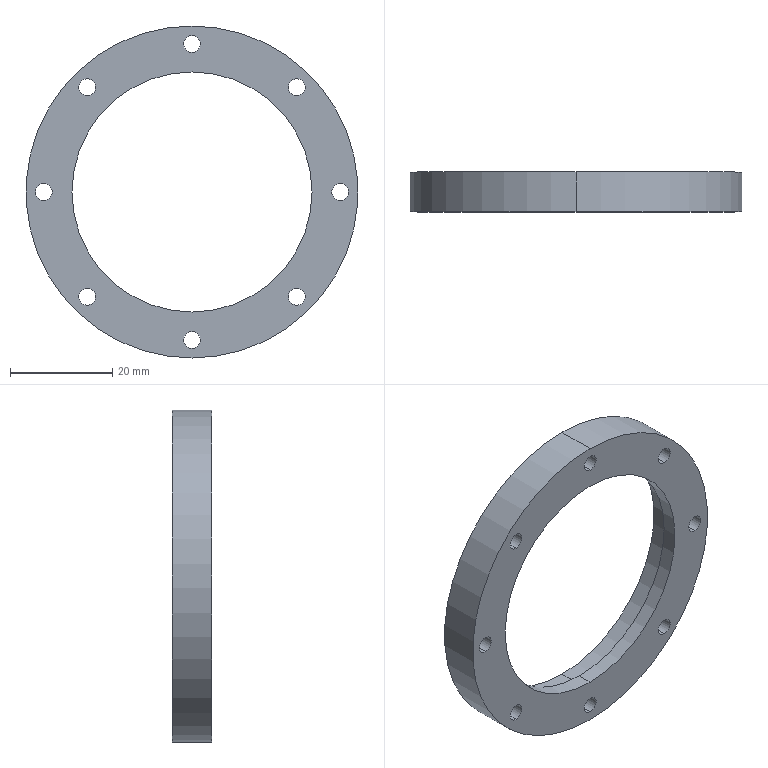Part | SolidWorks | features Extrusion 1, HoleWzd 1, ICE 1 | 1 solid | 25 faces | box 65 x 7.8 x 65 mm | volume 10339 mm3 | cylinder 22 | plane 3 | commonest cylinder face diameters 3.3 x16 47 x2 51 x2 65 x2
STEP:
#1=CARTESIAN_POINT('',(0.,0.,-30.65));
#2=VERTEX_POINT('',#1);
#3=CARTESIAN_POINT('',(0.,0.,-27.35));
#4=VERTEX_POINT('',#3);
#5=CARTESIAN_POINT('',(0.,0.,-29.));
#6=DIRECTION('',(0.,1.,0.));
#7=DIRECTION('',(0.,0.,1.));
#8=AXIS2_PLACEMENT_3D('',#5,#6,#7);
#9=CIRCLE('',#8,1.65);
#10=EDGE_CURVE('',#2,#4,#9,.T.);
#11=ORIENTED_EDGE('',*,*,#10,.F.);
#12=CARTESIAN_POINT('',(0.,7.8,-30.65));
#13=VERTEX_POINT('',#12);
#14=CARTESIAN_POINT('',(0.,7.8,-30.65));
#15=DIRECTION('',(0.,1.,0.));
#16=VECTOR('',#15,1000.);
#17=LINE('',#14,#16);
#18=EDGE_CURVE('',#2,#13,#17,.T.);
#19=ORIENTED_EDGE('',*,*,#18,.T.);
#20=CARTESIAN_POINT('',(0.,7.8,-27.35));
#21=VERTEX_POINT('',#20);
#22=CARTESIAN_POINT('',(0.,7.8,-29.));
#23=DIRECTION('',(0.,1.,0.));
#24=DIRECTION('',(0.,0.,1.));
#25=AXIS2_PLACEMENT_3D('',#22,#23,#24);
#26=CIRCLE('',#25,1.65);
#27=EDGE_CURVE('',#13,#21,#26,.T.);
#28=ORIENTED_EDGE('',*,*,#27,.T.);
#29=CARTESIAN_POINT('',(0.,7.8,-27.35));
#30=DIRECTION('',(0.,1.,0.));
#31=VECTOR('',#30,1000.);
#32=LINE('',#29,#31);
#33=EDGE_CURVE('',#4,#21,#32,.T.);
#34=ORIENTED_EDGE('',*,*,#33,.F.);
#35=EDGE_LOOP('',(#11,#19,#28,#34));
#36=FACE_OUTER_BOUND('',#35,.T.);
#37=CARTESIAN_POINT('',(0.,7.8,-29.));
#38=DIRECTION('',(0.,1.,0.));
#39=DIRECTION('',(0.,0.,1.));
#40=AXIS2_PLACEMENT_3D('',#37,#38,#39);
#41=CYLINDRICAL_SURFACE('',#40,1.65);
#42=ADVANCED_FACE('',(#36),#41,.F.);
#43=CARTESIAN_POINT('',(20.506,0.,-22.156));
#44=VERTEX_POINT('',#43);
#45=CARTESIAN_POINT('',(20.506,0.,-18.856));
#46=VERTEX_POINT('',#45);
#47=CARTESIAN_POINT('',(20.506,0.,-20.506));
#48=DIRECTION('',(0.,1.,0.));
#49=DIRECTION('',(0.,0.,1.));
#50=AXIS2_PLACEMENT_3D('',#47,#48,#49);
#51=CIRCLE('',#50,1.65);
#52=EDGE_CURVE('',#44,#46,#51,.T.);
#53=ORIENTED_EDGE('',*,*,#52,.F.);
#54=CARTESIAN_POINT('',(20.506,7.8,-22.156));
#55=VERTEX_POINT('',#54);
#56=CARTESIAN_POINT('',(20.506,7.8,-22.156));
#57=DIRECTION('',(0.,1.,0.));
#58=VECTOR('',#57,1000.);
#59=LINE('',#56,#58);
#60=EDGE_CURVE('',#44,#55,#59,.T.);
#61=ORIENTED_EDGE('',*,*,#60,.T.);
#62=CARTESIAN_POINT('',(20.506,7.8,-18.856));
#63=VERTEX_POINT('',#62);
#64=CARTESIAN_POINT('',(20.506,7.8,-20.506));
#65=DIRECTION('',(0.,1.,0.));
#66=DIRECTION('',(0.,0.,1.));
#67=AXIS2_PLACEMENT_3D('',#64,#65,#66);
#68=CIRCLE('',#67,1.65);
#69=EDGE_CURVE('',#55,#63,#68,.T.);
#70=ORIENTED_EDGE('',*,*,#69,.T.);
#71=CARTESIAN_POINT('',(20.506,7.8,-18.856));
#72=DIRECTION('',(0.,1.,0.));
#73=VECTOR('',#72,1000.);
#74=LINE('',#71,#73);
#75=EDGE_CURVE('',#46,#63,#74,.T.);
#76=ORIENTED_EDGE('',*,*,#75,.F.);
#77=EDGE_LOOP('',(#53,#61,#70,#76));
#78=FACE_OUTER_BOUND('',#77,.T.);
#79=CARTESIAN_POINT('',(20.506,7.8,-20.506));
#80=DIRECTION('',(0.,1.,0.));
#81=DIRECTION('',(0.,0.,1.));
#82=AXIS2_PLACEMENT_3D('',#79,#80,#81);
#83=CYLINDRICAL_SURFACE('',#82,1.65);
#84=ADVANCED_FACE('',(#78),#83,.F.);
#85=CARTESIAN_POINT('',(29.,0.,-1.65));
#86=VERTEX_POINT('',#85);
#87=CARTESIAN_POINT('',(29.,0.,1.65));
#88=VERTEX_POINT('',#87);
#89=CARTESIAN_POINT('',(29.,0.,0.));
#90=DIRECTION('',(0.,1.,0.));
#91=DIRECTION('',(0.,0.,1.));
#92=AXIS2_PLACEMENT_3D('',#89,#90,#91);
#93=CIRCLE('',#92,1.65);
#94=EDGE_CURVE('',#86,#88,#93,.T.);
#95=ORIENTED_EDGE('',*,*,#94,.F.);
#96=CARTESIAN_POINT('',(29.,7.8,-1.65));
#97=VERTEX_POINT('',#96);
#98=CARTESIAN_POINT('',(29.,7.8,-1.65));
#99=DIRECTION('',(0.,1.,0.));
#100=VECTOR('',#99,1000.);
#101=LINE('',#98,#100);
#102=EDGE_CURVE('',#86,#97,#101,.T.);
#103=ORIENTED_EDGE('',*,*,#102,.T.);
#104=CARTESIAN_POINT('',(29.,7.8,1.65));
#105=VERTEX_POINT('',#104);
#106=CARTESIAN_POINT('',(29.,7.8,0.));
#107=DIRECTION('',(0.,1.,0.));
#108=DIRECTION('',(0.,0.,1.));
#109=AXIS2_PLACEMENT_3D('',#106,#107,#108);
#110=CIRCLE('',#109,1.65);
#111=EDGE_CURVE('',#97,#105,#110,.T.);
#112=ORIENTED_EDGE('',*,*,#111,.T.);
#113=CARTESIAN_POINT('',(29.,7.8,1.65));
#114=DIRECTION('',(0.,1.,0.));
#115=VECTOR('',#114,1000.);
#116=LINE('',#113,#115);
#117=EDGE_CURVE('',#88,#105,#116,.T.);
#118=ORIENTED_EDGE('',*,*,#117,.F.);
#119=EDGE_LOOP('',(#95,#103,#112,#118));
#120=FACE_OUTER_BOUND('',#119,.T.);
#121=CARTESIAN_POINT('',(29.,7.8,0.));
#122=DIRECTION('',(0.,1.,0.));
#123=DIRECTION('',(0.,0.,1.));
#124=AXIS2_PLACEMENT_3D('',#121,#122,#123);
#125=CYLINDRICAL_SURFACE('',#124,1.65);
#126=ADVANCED_FACE('',(#120),#125,.F.);
#127=CARTESIAN_POINT('',(20.506,0.,18.856));
#128=VERTEX_POINT('',#127);
#129=CARTESIAN_POINT('',(20.506,0.,22.156));
#130=VERTEX_POINT('',#129);
#131=CARTESIAN_POINT('',(20.506,0.,20.506));
#132=DIRECTION('',(0.,1.,0.));
#133=DIRECTION('',(0.,0.,1.));
#134=AXIS2_PLACEMENT_3D('',#131,#132,#133);
#135=CIRCLE('',#134,1.65);
#136=EDGE_CURVE('',#128,#130,#135,.T.);
#137=ORIENTED_EDGE('',*,*,#136,.F.);
#138=CARTESIAN_POINT('',(20.506,7.8,18.856));
#139=VERTEX_POINT('',#138);
#140=CARTESIAN_POINT('',(20.506,7.8,18.856));
#141=DIRECTION('',(0.,1.,0.));
#142=VECTOR('',#141,1000.);
#143=LINE('',#140,#142);
#144=EDGE_CURVE('',#128,#139,#143,.T.);
#145=ORIENTED_EDGE('',*,*,#144,.T.);
#146=CARTESIAN_POINT('',(20.506,7.8,22.156));
#147=VERTEX_POINT('',#146);
#148=CARTESIAN_POINT('',(20.506,7.8,20.506));
#149=DIRECTION('',(0.,1.,0.));
#150=DIRECTION('',(0.,0.,1.));
#151=AXIS2_PLACEMENT_3D('',#148,#149,#150);
#152=CIRCLE('',#151,1.65);
#153=EDGE_CURVE('',#139,#147,#152,.T.);
#154=ORIENTED_EDGE('',*,*,#153,.T.);
#155=CARTESIAN_POINT('',(20.506,7.8,22.156));
#156=DIRECTION('',(0.,1.,0.));
#157=VECTOR('',#156,1000.);
#158=LINE('',#155,#157);
#159=EDGE_CURVE('',#130,#147,#158,.T.);
#160=ORIENTED_EDGE('',*,*,#159,.F.);
#161=EDGE_LOOP('',(#137,#145,#154,#160));
#162=FACE_OUTER_BOUND('',#161,.T.);
#163=CARTESIAN_POINT('',(20.506,7.8,20.506));
#164=DIRECTION('',(0.,1.,0.));
#165=DIRECTION('',(0.,0.,1.));
#166=AXIS2_PLACEMENT_3D('',#163,#164,#165);
#167=CYLINDRICAL_SURFACE('',#166,1.65);
#168=ADVANCED_FACE('',(#162),#167,.F.);
#169=CARTESIAN_POINT('',(0.,0.,27.35));
#170=VERTEX_POINT('',#169);
#171=CARTESIAN_POINT('',(0.,0.,30.65));
#172=VERTEX_POINT('',#171);
#173=CARTESIAN_POINT('',(0.,0.,29.));
#174=DIRECTION('',(0.,1.,0.));
#175=DIRECTION('',(0.,0.,1.));
#176=AXIS2_PLACEMENT_3D('',#173,#174,#175);
#177=CIRCLE('',#176,1.65);
#178=EDGE_CURVE('',#170,#172,#177,.T.);
#179=ORIENTED_EDGE('',*,*,#178,.F.);
#180=CARTESIAN_POINT('',(0.,7.8,27.35));
#181=VERTEX_POINT('',#180);
#182=CARTESIAN_POINT('',(0.,7.8,27.35));
#183=DIRECTION('',(0.,1.,0.));
#184=VECTOR('',#183,1000.);
#185=LINE('',#182,#184);
#186=EDGE_CURVE('',#170,#181,#185,.T.);
#187=ORIENTED_EDGE('',*,*,#186,.T.);
#188=CARTESIAN_POINT('',(0.,7.8,30.65));
#189=VERTEX_POINT('',#188);
#190=CARTESIAN_POINT('',(0.,7.8,29.));
#191=DIRECTION('',(0.,1.,0.));
#192=DIRECTION('',(0.,0.,1.));
#193=AXIS2_PLACEMENT_3D('',#190,#191,#192);
#194=CIRCLE('',#193,1.65);
#195=EDGE_CURVE('',#181,#189,#194,.T.);
#196=ORIENTED_EDGE('',*,*,#195,.T.);
#197=CARTESIAN_POINT('',(0.,7.8,30.65));
#198=DIRECTION('',(0.,1.,0.));
#199=VECTOR('',#198,1000.);
#200=LINE('',#197,#199);
#201=EDGE_CURVE('',#172,#189,#200,.T.);
#202=ORIENTED_EDGE('',*,*,#201,.F.);
#203=EDGE_LOOP('',(#179,#187,#196,#202));
#204=FACE_OUTER_BOUND('',#203,.T.);
#205=CARTESIAN_POINT('',(0.,7.8,29.));
#206=DIRECTION('',(0.,1.,0.));
#207=DIRECTION('',(0.,0.,1.));
#208=AXIS2_PLACEMENT_3D('',#205,#206,#207);
#209=CYLINDRICAL_SURFACE('',#208,1.65);
#210=ADVANCED_FACE('',(#204),#209,.F.);
#211=CARTESIAN_POINT('',(-20.506,0.,18.856));
#212=VERTEX_POINT('',#211);
#213=CARTESIAN_POINT('',(-20.506,0.,22.156));
#214=VERTEX_POINT('',#213);
#215=CARTESIAN_POINT('',(-20.506,0.,20.506));
#216=DIRECTION('',(0.,1.,0.));
#217=DIRECTION('',(0.,0.,1.));
#218=AXIS2_PLACEMENT_3D('',#215,#216,#217);
#219=CIRCLE('',#218,1.65);
#220=EDGE_CURVE('',#212,#214,#219,.T.);
#221=ORIENTED_EDGE('',*,*,#220,.F.);
#222=CARTESIAN_POINT('',(-20.506,7.8,18.856));
#223=VERTEX_POINT('',#222);
#224=CARTESIAN_POINT('',(-20.506,7.8,18.856));
#225=DIRECTION('',(0.,1.,0.));
#226=VECTOR('',#225,1000.);
#227=LINE('',#224,#226);
#228=EDGE_CURVE('',#212,#223,#227,.T.);
#229=ORIENTED_EDGE('',*,*,#228,.T.);
#230=CARTESIAN_POINT('',(-20.506,7.8,22.156));
#231=VERTEX_POINT('',#230);
#232=CARTESIAN_POINT('',(-20.506,7.8,20.506));
#233=DIRECTION('',(0.,1.,0.));
#234=DIRECTION('',(0.,0.,1.));
#235=AXIS2_PLACEMENT_3D('',#232,#233,#234);
#236=CIRCLE('',#235,1.65);
#237=EDGE_CURVE('',#223,#231,#236,.T.);
#238=ORIENTED_EDGE('',*,*,#237,.T.);
#239=CARTESIAN_POINT('',(-20.506,7.8,22.156));
#240=DIRECTION('',(0.,1.,0.));
#241=VECTOR('',#240,1000.);
#242=LINE('',#239,#241);
#243=EDGE_CURVE('',#214,#231,#242,.T.);
#244=ORIENTED_EDGE('',*,*,#243,.F.);
#245=EDGE_LOOP('',(#221,#229,#238,#244));
#246=FACE_OUTER_BOUND('',#245,.T.);
#247=CARTESIAN_POINT('',(-20.506,7.8,20.506));
#248=DIRECTION('',(0.,1.,0.));
#249=DIRECTION('',(0.,0.,1.));
#250=AXIS2_PLACEMENT_3D('',#247,#248,#249);
#251=CYLINDRICAL_SURFACE('',#250,1.65);
#252=ADVANCED_FACE('',(#246),#251,.F.);
#253=CARTESIAN_POINT('',(-29.,0.,-1.65));
#254=VERTEX_POINT('',#253);
#255=CARTESIAN_POINT('',(-29.,0.,1.65));
#256=VERTEX_POINT('',#255);
#257=CARTESIAN_POINT('',(-29.,0.,0.));
#258=DIRECTION('',(0.,1.,0.));
#259=DIRECTION('',(0.,0.,1.));
#260=AXIS2_PLACEMENT_3D('',#257,#258,#259);
#261=CIRCLE('',#260,1.65);
#262=EDGE_CURVE('',#254,#256,#261,.T.);
#263=ORIENTED_EDGE('',*,*,#262,.F.);
#264=CARTESIAN_POINT('',(-29.,7.8,-1.65));
#265=VERTEX_POINT('',#264);
#266=CARTESIAN_POINT('',(-29.,7.8,-1.65));
#267=DIRECTION('',(0.,1.,0.));
#268=VECTOR('',#267,1000.);
#269=LINE('',#266,#268);
#270=EDGE_CURVE('',#254,#265,#269,.T.);
#271=ORIENTED_EDGE('',*,*,#270,.T.);
#272=CARTESIAN_POINT('',(-29.,7.8,1.65));
#273=VERTEX_POINT('',#272);
#274=CARTESIAN_POINT('',(-29.,7.8,0.));
#275=DIRECTION('',(0.,1.,0.));
#276=DIRECTION('',(0.,0.,1.));
#277=AXIS2_PLACEMENT_3D('',#274,#275,#276);
#278=CIRCLE('',#277,1.65);
#279=EDGE_CURVE('',#265,#273,#278,.T.);
#280=ORIENTED_EDGE('',*,*,#279,.T.);
#281=CARTESIAN_POINT('',(-29.,7.8,1.65));
#282=DIRECTION('',(0.,1.,0.));
#283=VECTOR('',#282,1000.);
#284=LINE('',#281,#283);
#285=EDGE_CURVE('',#256,#273,#284,.T.);
#286=ORIENTED_EDGE('',*,*,#285,.F.);
#287=EDGE_LOOP('',(#263,#271,#280,#286));
#288=FACE_OUTER_BOUND('',#287,.T.);
#289=CARTESIAN_POINT('',(-29.,7.8,0.));
#290=DIRECTION('',(0.,1.,0.));
#291=DIRECTION('',(0.,0.,1.));
#292=AXIS2_PLACEMENT_3D('',#289,#290,#291);
#293=CYLINDRICAL_SURFACE('',#292,1.65);
#294=ADVANCED_FACE('',(#288),#293,.F.);
#295=CARTESIAN_POINT('',(-20.506,0.,-22.156));
#296=VERTEX_POINT('',#295);
#297=CARTESIAN_POINT('',(-20.506,0.,-18.856));
#298=VERTEX_POINT('',#297);
#299=CARTESIAN_POINT('',(-20.506,0.,-20.506));
#300=DIRECTION('',(0.,1.,0.));
#301=DIRECTION('',(0.,0.,1.));
#302=AXIS2_PLACEMENT_3D('',#299,#300,#301);
#303=CIRCLE('',#302,1.65);
#304=EDGE_CURVE('',#296,#298,#303,.T.);
#305=ORIENTED_EDGE('',*,*,#304,.F.);
#306=CARTESIAN_POINT('',(-20.506,7.8,-22.156));
#307=VERTEX_POINT('',#306);
#308=CARTESIAN_POINT('',(-20.506,7.8,-22.156));
#309=DIRECTION('',(0.,1.,0.));
#310=VECTOR('',#309,1000.);
#311=LINE('',#308,#310);
#312=EDGE_CURVE('',#296,#307,#311,.T.);
#313=ORIENTED_EDGE('',*,*,#312,.T.);
#314=CARTESIAN_POINT('',(-20.506,7.8,-18.856));
#315=VERTEX_POINT('',#314);
#316=CARTESIAN_POINT('',(-20.506,7.8,-20.506));
#317=DIRECTION('',(0.,1.,0.));
#318=DIRECTION('',(0.,0.,1.));
#319=AXIS2_PLACEMENT_3D('',#316,#317,#318);
#320=CIRCLE('',#319,1.65);
#321=EDGE_CURVE('',#307,#315,#320,.T.);
#322=ORIENTED_EDGE('',*,*,#321,.T.);
#323=CARTESIAN_POINT('',(-20.506,7.8,-18.856));
#324=DIRECTION('',(0.,1.,0.));
#325=VECTOR('',#324,1000.);
#326=LINE('',#323,#325);
#327=EDGE_CURVE('',#298,#315,#326,.T.);
#328=ORIENTED_EDGE('',*,*,#327,.F.);
#329=EDGE_LOOP('',(#305,#313,#322,#328));
#330=FACE_OUTER_BOUND('',#329,.T.);
#331=CARTESIAN_POINT('',(-20.506,7.8,-20.506));
#332=DIRECTION('',(0.,1.,0.));
#333=DIRECTION('',(0.,0.,1.));
#334=AXIS2_PLACEMENT_3D('',#331,#332,#333);
#335=CYLINDRICAL_SURFACE('',#334,1.65);
#336=ADVANCED_FACE('',(#330),#335,.F.);
#337=CARTESIAN_POINT('',(0.,7.8,-25.5));
#338=VERTEX_POINT('',#337);
#339=CARTESIAN_POINT('',(0.,7.8,25.5));
#340=VERTEX_POINT('',#339);
#341=CARTESIAN_POINT('',(0.,7.8,0.));
#342=DIRECTION('',(0.,1.,0.));
#343=DIRECTION('',(0.,0.,1.));
#344=AXIS2_PLACEMENT_3D('',#341,#342,#343);
#345=CIRCLE('',#344,25.5);
#346=EDGE_CURVE('',#338,#340,#345,.T.);
#347=ORIENTED_EDGE('',*,*,#346,.T.);
#348=CARTESIAN_POINT('',(0.,3.,25.5));
#349=VERTEX_POINT('',#348);
#350=CARTESIAN_POINT('',(0.,7.8,25.5));
#351=DIRECTION('',(0.,-1.,0.));
#352=VECTOR('',#351,1000.);
#353=LINE('',#350,#352);
#354=EDGE_CURVE('',#340,#349,#353,.T.);
#355=ORIENTED_EDGE('',*,*,#354,.T.);
#356=CARTESIAN_POINT('',(0.,3.,-25.5));
#357=VERTEX_POINT('',#356);
#358=CARTESIAN_POINT('',(0.,3.,0.));
#359=DIRECTION('',(0.,1.,0.));
#360=DIRECTION('',(0.,0.,1.));
#361=AXIS2_PLACEMENT_3D('',#358,#359,#360);
#362=CIRCLE('',#361,25.5);
#363=EDGE_CURVE('',#357,#349,#362,.T.);
#364=ORIENTED_EDGE('',*,*,#363,.F.);
#365=CARTESIAN_POINT('',(0.,7.8,-25.5));
#366=DIRECTION('',(0.,-1.,0.));
#367=VECTOR('',#366,1000.);
#368=LINE('',#365,#367);
#369=EDGE_CURVE('',#338,#357,#368,.T.);
#370=ORIENTED_EDGE('',*,*,#369,.F.);
#371=EDGE_LOOP('',(#347,#355,#364,#370));
#372=FACE_OUTER_BOUND('',#371,.T.);
#373=CARTESIAN_POINT('',(0.,7.8,0.));
#374=DIRECTION('',(0.,-1.,0.));
#375=DIRECTION('',(0.,0.,-1.));
#376=AXIS2_PLACEMENT_3D('',#373,#374,#375);
#377=CYLINDRICAL_SURFACE('',#376,25.5);
#378=ADVANCED_FACE('',(#372),#377,.F.);
#379=CARTESIAN_POINT('',(0.,3.,-23.5));
#380=VERTEX_POINT('',#379);
#381=CARTESIAN_POINT('',(0.,3.,23.5));
#382=VERTEX_POINT('',#381);
#383=CARTESIAN_POINT('',(0.,3.,0.));
#384=DIRECTION('',(0.,1.,0.));
#385=DIRECTION('',(0.,0.,1.));
#386=AXIS2_PLACEMENT_3D('',#383,#384,#385);
#387=CIRCLE('',#386,23.5);
#388=EDGE_CURVE('',#380,#382,#387,.T.);
#389=ORIENTED_EDGE('',*,*,#388,.T.);
#390=CARTESIAN_POINT('',(0.,0.,23.5));
#391=VERTEX_POINT('',#390);
#392=CARTESIAN_POINT('',(0.,3.,23.5));
#393=DIRECTION('',(0.,-1.,0.));
#394=VECTOR('',#393,1000.);
#395=LINE('',#392,#394);
#396=EDGE_CURVE('',#382,#391,#395,.T.);
#397=ORIENTED_EDGE('',*,*,#396,.T.);
#398=CARTESIAN_POINT('',(0.,0.,-23.5));
#399=VERTEX_POINT('',#398);
#400=CARTESIAN_POINT('',(0.,0.,0.));
#401=DIRECTION('',(0.,1.,0.));
#402=DIRECTION('',(0.,0.,1.));
#403=AXIS2_PLACEMENT_3D('',#400,#401,#402);
#404=CIRCLE('',#403,23.5);
#405=EDGE_CURVE('',#399,#391,#404,.T.);
#406=ORIENTED_EDGE('',*,*,#405,.F.);
#407=CARTESIAN_POINT('',(0.,3.,-23.5));
#408=DIRECTION('',(0.,-1.,0.));
#409=VECTOR('',#408,1000.);
#410=LINE('',#407,#409);
#411=EDGE_CURVE('',#380,#399,#410,.T.);
#412=ORIENTED_EDGE('',*,*,#411,.F.);
#413=EDGE_LOOP('',(#389,#397,#406,#412));
#414=FACE_OUTER_BOUND('',#413,.T.);
#415=CARTESIAN_POINT('',(0.,3.,0.));
#416=DIRECTION('',(0.,-1.,0.));
#417=DIRECTION('',(0.,0.,-1.));
#418=AXIS2_PLACEMENT_3D('',#415,#416,#417);
#419=CYLINDRICAL_SURFACE('',#418,23.5);
#420=ADVANCED_FACE('',(#414),#419,.F.);
#421=CARTESIAN_POINT('',(0.,7.8,32.5));
#422=VERTEX_POINT('',#421);
#423=CARTESIAN_POINT('',(0.,7.8,-32.5));
#424=VERTEX_POINT('',#423);
#425=CARTESIAN_POINT('',(0.,7.8,0.));
#426=DIRECTION('',(0.,1.,0.));
#427=DIRECTION('',(0.,0.,1.));
#428=AXIS2_PLACEMENT_3D('',#425,#426,#427);
#429=CIRCLE('',#428,32.5);
#430=EDGE_CURVE('',#422,#424,#429,.T.);
#431=ORIENTED_EDGE('',*,*,#430,.F.);
#432=CARTESIAN_POINT('',(0.,0.,32.5));
#433=VERTEX_POINT('',#432);
#434=CARTESIAN_POINT('',(0.,3.,32.5));
#435=DIRECTION('',(0.,-1.,0.));
#436=VECTOR('',#435,1000.);
#437=LINE('',#434,#436);
#438=EDGE_CURVE('',#422,#433,#437,.T.);
#439=ORIENTED_EDGE('',*,*,#438,.T.);
#440=CARTESIAN_POINT('',(0.,0.,-32.5));
#441=VERTEX_POINT('',#440);
#442=CARTESIAN_POINT('',(0.,0.,0.));
#443=DIRECTION('',(0.,1.,0.));
#444=DIRECTION('',(0.,0.,1.));
#445=AXIS2_PLACEMENT_3D('',#442,#443,#444);
#446=CIRCLE('',#445,32.5);
#447=EDGE_CURVE('',#433,#441,#446,.T.);
#448=ORIENTED_EDGE('',*,*,#447,.T.);
#449=CARTESIAN_POINT('',(0.,3.,-32.5));
#450=DIRECTION('',(0.,-1.,0.));
#451=VECTOR('',#450,1000.);
#452=LINE('',#449,#451);
#453=EDGE_CURVE('',#424,#441,#452,.T.);
#454=ORIENTED_EDGE('',*,*,#453,.F.);
#455=EDGE_LOOP('',(#431,#439,#448,#454));
#456=FACE_OUTER_BOUND('',#455,.T.);
#457=CARTESIAN_POINT('',(0.,3.,0.));
#458=DIRECTION('',(0.,-1.,0.));
#459=DIRECTION('',(0.,0.,-1.));
#460=AXIS2_PLACEMENT_3D('',#457,#458,#459);
#461=CYLINDRICAL_SURFACE('',#460,32.5);
#462=ADVANCED_FACE('',(#456),#461,.T.);
#463=ORIENTED_EDGE('',*,*,#388,.F.);
#464=CARTESIAN_POINT('',(0.,3.,0.));
#465=DIRECTION('',(0.,1.,0.));
#466=DIRECTION('',(0.,0.,1.));
#467=AXIS2_PLACEMENT_3D('',#464,#465,#466);
#468=CIRCLE('',#467,23.5);
#469=EDGE_CURVE('',#382,#380,#468,.T.);
#470=ORIENTED_EDGE('',*,*,#469,.F.);
#471=EDGE_LOOP('',(#463,#470));
#472=FACE_BOUND('',#471,.T.);
#473=ORIENTED_EDGE('',*,*,#363,.T.);
#474=CARTESIAN_POINT('',(0.,3.,0.));
#475=DIRECTION('',(0.,1.,0.));
#476=DIRECTION('',(0.,0.,1.));
#477=AXIS2_PLACEMENT_3D('',#474,#475,#476);
#478=CIRCLE('',#477,25.5);
#479=EDGE_CURVE('',#349,#357,#478,.T.);
#480=ORIENTED_EDGE('',*,*,#479,.T.);
#481=EDGE_LOOP('',(#473,#480));
#482=FACE_OUTER_BOUND('',#481,.T.);
#483=CARTESIAN_POINT('',(0.,3.,0.));
#484=DIRECTION('',(0.,1.,0.));
#485=DIRECTION('',(0.,0.,1.));
#486=AXIS2_PLACEMENT_3D('',#483,#484,#485);
#487=PLANE('',#486);
#488=ADVANCED_FACE('',(#472,#482),#487,.T.);
#489=CARTESIAN_POINT('',(0.,0.,-29.));
#490=DIRECTION('',(0.,1.,0.));
#491=DIRECTION('',(0.,0.,1.));
#492=AXIS2_PLACEMENT_3D('',#489,#490,#491);
#493=CIRCLE('',#492,1.65);
#494=EDGE_CURVE('',#4,#2,#493,.T.);
#495=ORIENTED_EDGE('',*,*,#494,.T.);
#496=ORIENTED_EDGE('',*,*,#10,.T.);
#497=EDGE_LOOP('',(#495,#496));
#498=FACE_BOUND('',#497,.T.);
#499=CARTESIAN_POINT('',(20.506,0.,-20.506));
#500=DIRECTION('',(0.,1.,0.));
#501=DIRECTION('',(0.,0.,1.));
#502=AXIS2_PLACEMENT_3D('',#499,#500,#501);
#503=CIRCLE('',#502,1.65);
#504=EDGE_CURVE('',#46,#44,#503,.T.);
#505=ORIENTED_EDGE('',*,*,#504,.T.);
#506=ORIENTED_EDGE('',*,*,#52,.T.);
#507=EDGE_LOOP('',(#505,#506));
#508=FACE_BOUND('',#507,.T.);
#509=CARTESIAN_POINT('',(29.,0.,0.));
#510=DIRECTION('',(0.,1.,0.));
#511=DIRECTION('',(0.,0.,1.));
#512=AXIS2_PLACEMENT_3D('',#509,#510,#511);
#513=CIRCLE('',#512,1.65);
#514=EDGE_CURVE('',#88,#86,#513,.T.);
#515=ORIENTED_EDGE('',*,*,#514,.T.);
#516=ORIENTED_EDGE('',*,*,#94,.T.);
#517=EDGE_LOOP('',(#515,#516));
#518=FACE_BOUND('',#517,.T.);
#519=CARTESIAN_POINT('',(20.506,0.,20.506));
#520=DIRECTION('',(0.,1.,0.));
#521=DIRECTION('',(0.,0.,1.));
#522=AXIS2_PLACEMENT_3D('',#519,#520,#521);
#523=CIRCLE('',#522,1.65);
#524=EDGE_CURVE('',#130,#128,#523,.T.);
#525=ORIENTED_EDGE('',*,*,#524,.T.);
#526=ORIENTED_EDGE('',*,*,#136,.T.);
#527=EDGE_LOOP('',(#525,#526));
#528=FACE_BOUND('',#527,.T.);
#529=CARTESIAN_POINT('',(0.,0.,29.));
#530=DIRECTION('',(0.,1.,0.));
#531=DIRECTION('',(0.,0.,1.));
#532=AXIS2_PLACEMENT_3D('',#529,#530,#531);
#533=CIRCLE('',#532,1.65);
#534=EDGE_CURVE('',#172,#170,#533,.T.);
#535=ORIENTED_EDGE('',*,*,#534,.T.);
#536=ORIENTED_EDGE('',*,*,#178,.T.);
#537=EDGE_LOOP('',(#535,#536));
#538=FACE_BOUND('',#537,.T.);
#539=CARTESIAN_POINT('',(-20.506,0.,20.506));
#540=DIRECTION('',(0.,1.,0.));
#541=DIRECTION('',(0.,0.,1.));
#542=AXIS2_PLACEMENT_3D('',#539,#540,#541);
#543=CIRCLE('',#542,1.65);
#544=EDGE_CURVE('',#214,#212,#543,.T.);
#545=ORIENTED_EDGE('',*,*,#544,.T.);
#546=ORIENTED_EDGE('',*,*,#220,.T.);
#547=EDGE_LOOP('',(#545,#546));
#548=FACE_BOUND('',#547,.T.);
#549=CARTESIAN_POINT('',(-29.,0.,0.));
#550=DIRECTION('',(0.,1.,0.));
#551=DIRECTION('',(0.,0.,1.));
#552=AXIS2_PLACEMENT_3D('',#549,#550,#551);
#553=CIRCLE('',#552,1.65);
#554=EDGE_CURVE('',#256,#254,#553,.T.);
#555=ORIENTED_EDGE('',*,*,#554,.T.);
#556=ORIENTED_EDGE('',*,*,#262,.T.);
#557=EDGE_LOOP('',(#555,#556));
#558=FACE_BOUND('',#557,.T.);
#559=CARTESIAN_POINT('',(-20.506,0.,-20.506));
#560=DIRECTION('',(0.,1.,0.));
#561=DIRECTION('',(0.,0.,1.));
#562=AXIS2_PLACEMENT_3D('',#559,#560,#561);
#563=CIRCLE('',#562,1.65);
#564=EDGE_CURVE('',#298,#296,#563,.T.);
#565=ORIENTED_EDGE('',*,*,#564,.T.);
#566=ORIENTED_EDGE('',*,*,#304,.T.);
#567=EDGE_LOOP('',(#565,#566));
#568=FACE_BOUND('',#567,.T.);
#569=CARTESIAN_POINT('',(0.,0.,0.));
#570=DIRECTION('',(0.,1.,0.));
#571=DIRECTION('',(0.,0.,1.));
#572=AXIS2_PLACEMENT_3D('',#569,#570,#571);
#573=CIRCLE('',#572,32.5);
#574=EDGE_CURVE('',#441,#433,#573,.T.);
#575=ORIENTED_EDGE('',*,*,#574,.F.);
#576=ORIENTED_EDGE('',*,*,#447,.F.);
#577=EDGE_LOOP('',(#575,#576));
#578=FACE_OUTER_BOUND('',#577,.T.);
#579=ORIENTED_EDGE('',*,*,#405,.T.);
#580=CARTESIAN_POINT('',(0.,0.,0.));
#581=DIRECTION('',(0.,1.,0.));
#582=DIRECTION('',(0.,0.,1.));
#583=AXIS2_PLACEMENT_3D('',#580,#581,#582);
#584=CIRCLE('',#583,23.5);
#585=EDGE_CURVE('',#391,#399,#584,.T.);
#586=ORIENTED_EDGE('',*,*,#585,.T.);
#587=EDGE_LOOP('',(#579,#586));
#588=FACE_BOUND('',#587,.T.);
#589=CARTESIAN_POINT('',(0.,0.,0.));
#590=DIRECTION('',(0.,1.,0.));
#591=DIRECTION('',(0.,0.,1.));
#592=AXIS2_PLACEMENT_3D('',#589,#590,#591);
#593=PLANE('',#592);
#594=ADVANCED_FACE('',(#498,#508,#518,#528,#538,#548,#558,#568,#578,#588),#593,.F.);
#595=ORIENTED_EDGE('',*,*,#438,.F.);
#596=CARTESIAN_POINT('',(0.,7.8,0.));
#597=DIRECTION('',(0.,1.,0.));
#598=DIRECTION('',(0.,0.,1.));
#599=AXIS2_PLACEMENT_3D('',#596,#597,#598);
#600=CIRCLE('',#599,32.5);
#601=EDGE_CURVE('',#424,#422,#600,.T.);
#602=ORIENTED_EDGE('',*,*,#601,.F.);
#603=ORIENTED_EDGE('',*,*,#453,.T.);
#604=ORIENTED_EDGE('',*,*,#574,.T.);
#605=EDGE_LOOP('',(#595,#602,#603,#604));
#606=FACE_OUTER_BOUND('',#605,.T.);
#607=CARTESIAN_POINT('',(0.,3.,0.));
#608=DIRECTION('',(0.,-1.,0.));
#609=DIRECTION('',(0.,0.,-1.));
#610=AXIS2_PLACEMENT_3D('',#607,#608,#609);
#611=CYLINDRICAL_SURFACE('',#610,32.5);
#612=ADVANCED_FACE('',(#606),#611,.T.);
#613=ORIENTED_EDGE('',*,*,#396,.F.);
#614=ORIENTED_EDGE('',*,*,#469,.T.);
#615=ORIENTED_EDGE('',*,*,#411,.T.);
#616=ORIENTED_EDGE('',*,*,#585,.F.);
#617=EDGE_LOOP('',(#613,#614,#615,#616));
#618=FACE_OUTER_BOUND('',#617,.T.);
#619=CARTESIAN_POINT('',(0.,3.,0.));
#620=DIRECTION('',(0.,-1.,0.));
#621=DIRECTION('',(0.,0.,-1.));
#622=AXIS2_PLACEMENT_3D('',#619,#620,#621);
#623=CYLINDRICAL_SURFACE('',#622,23.5);
#624=ADVANCED_FACE('',(#618),#623,.F.);
#625=CARTESIAN_POINT('',(0.,7.8,-29.));
#626=DIRECTION('',(0.,1.,0.));
#627=DIRECTION('',(0.,0.,1.));
#628=AXIS2_PLACEMENT_3D('',#625,#626,#627);
#629=CIRCLE('',#628,1.65);
#630=EDGE_CURVE('',#21,#13,#629,.T.);
#631=ORIENTED_EDGE('',*,*,#630,.F.);
#632=ORIENTED_EDGE('',*,*,#27,.F.);
#633=EDGE_LOOP('',(#631,#632));
#634=FACE_BOUND('',#633,.T.);
#635=CARTESIAN_POINT('',(20.506,7.8,-20.506));
#636=DIRECTION('',(0.,1.,0.));
#637=DIRECTION('',(0.,0.,1.));
#638=AXIS2_PLACEMENT_3D('',#635,#636,#637);
#639=CIRCLE('',#638,1.65);
#640=EDGE_CURVE('',#63,#55,#639,.T.);
#641=ORIENTED_EDGE('',*,*,#640,.F.);
#642=ORIENTED_EDGE('',*,*,#69,.F.);
#643=EDGE_LOOP('',(#641,#642));
#644=FACE_BOUND('',#643,.T.);
#645=CARTESIAN_POINT('',(29.,7.8,0.));
#646=DIRECTION('',(0.,1.,0.));
#647=DIRECTION('',(0.,0.,1.));
#648=AXIS2_PLACEMENT_3D('',#645,#646,#647);
#649=CIRCLE('',#648,1.65);
#650=EDGE_CURVE('',#105,#97,#649,.T.);
#651=ORIENTED_EDGE('',*,*,#650,.F.);
#652=ORIENTED_EDGE('',*,*,#111,.F.);
#653=EDGE_LOOP('',(#651,#652));
#654=FACE_BOUND('',#653,.T.);
#655=CARTESIAN_POINT('',(20.506,7.8,20.506));
#656=DIRECTION('',(0.,1.,0.));
#657=DIRECTION('',(0.,0.,1.));
#658=AXIS2_PLACEMENT_3D('',#655,#656,#657);
#659=CIRCLE('',#658,1.65);
#660=EDGE_CURVE('',#147,#139,#659,.T.);
#661=ORIENTED_EDGE('',*,*,#660,.F.);
#662=ORIENTED_EDGE('',*,*,#153,.F.);
#663=EDGE_LOOP('',(#661,#662));
#664=FACE_BOUND('',#663,.T.);
#665=CARTESIAN_POINT('',(0.,7.8,29.));
#666=DIRECTION('',(0.,1.,0.));
#667=DIRECTION('',(0.,0.,1.));
#668=AXIS2_PLACEMENT_3D('',#665,#666,#667);
#669=CIRCLE('',#668,1.65);
#670=EDGE_CURVE('',#189,#181,#669,.T.);
#671=ORIENTED_EDGE('',*,*,#670,.F.);
#672=ORIENTED_EDGE('',*,*,#195,.F.);
#673=EDGE_LOOP('',(#671,#672));
#674=FACE_BOUND('',#673,.T.);
#675=CARTESIAN_POINT('',(-20.506,7.8,20.506));
#676=DIRECTION('',(0.,1.,0.));
#677=DIRECTION('',(0.,0.,1.));
#678=AXIS2_PLACEMENT_3D('',#675,#676,#677);
#679=CIRCLE('',#678,1.65);
#680=EDGE_CURVE('',#231,#223,#679,.T.);
#681=ORIENTED_EDGE('',*,*,#680,.F.);
#682=ORIENTED_EDGE('',*,*,#237,.F.);
#683=EDGE_LOOP('',(#681,#682));
#684=FACE_BOUND('',#683,.T.);
#685=CARTESIAN_POINT('',(-29.,7.8,0.));
#686=DIRECTION('',(0.,1.,0.));
#687=DIRECTION('',(0.,0.,1.));
#688=AXIS2_PLACEMENT_3D('',#685,#686,#687);
#689=CIRCLE('',#688,1.65);
#690=EDGE_CURVE('',#273,#265,#689,.T.);
#691=ORIENTED_EDGE('',*,*,#690,.F.);
#692=ORIENTED_EDGE('',*,*,#279,.F.);
#693=EDGE_LOOP('',(#691,#692));
#694=FACE_BOUND('',#693,.T.);
#695=CARTESIAN_POINT('',(-20.506,7.8,-20.506));
#696=DIRECTION('',(0.,1.,0.));
#697=DIRECTION('',(0.,0.,1.));
#698=AXIS2_PLACEMENT_3D('',#695,#696,#697);
#699=CIRCLE('',#698,1.65);
#700=EDGE_CURVE('',#315,#307,#699,.T.);
#701=ORIENTED_EDGE('',*,*,#700,.F.);
#702=ORIENTED_EDGE('',*,*,#321,.F.);
#703=EDGE_LOOP('',(#701,#702));
#704=FACE_BOUND('',#703,.T.);
#705=ORIENTED_EDGE('',*,*,#601,.T.);
#706=ORIENTED_EDGE('',*,*,#430,.T.);
#707=EDGE_LOOP('',(#705,#706));
#708=FACE_OUTER_BOUND('',#707,.T.);
#709=ORIENTED_EDGE('',*,*,#346,.F.);
#710=CARTESIAN_POINT('',(0.,7.8,0.));
#711=DIRECTION('',(0.,1.,0.));
#712=DIRECTION('',(0.,0.,1.));
#713=AXIS2_PLACEMENT_3D('',#710,#711,#712);
#714=CIRCLE('',#713,25.5);
#715=EDGE_CURVE('',#340,#338,#714,.T.);
#716=ORIENTED_EDGE('',*,*,#715,.F.);
#717=EDGE_LOOP('',(#709,#716));
#718=FACE_BOUND('',#717,.T.);
#719=CARTESIAN_POINT('',(0.,7.8,0.));
#720=DIRECTION('',(0.,1.,0.));
#721=DIRECTION('',(0.,0.,1.));
#722=AXIS2_PLACEMENT_3D('',#719,#720,#721);
#723=PLANE('',#722);
#724=ADVANCED_FACE('',(#634,#644,#654,#664,#674,#684,#694,#704,#708,#718),#723,.T.);
#725=ORIENTED_EDGE('',*,*,#354,.F.);
#726=ORIENTED_EDGE('',*,*,#715,.T.);
#727=ORIENTED_EDGE('',*,*,#369,.T.);
#728=ORIENTED_EDGE('',*,*,#479,.F.);
#729=EDGE_LOOP('',(#725,#726,#727,#728));
#730=FACE_OUTER_BOUND('',#729,.T.);
#731=CARTESIAN_POINT('',(0.,7.8,0.));
#732=DIRECTION('',(0.,-1.,0.));
#733=DIRECTION('',(0.,0.,-1.));
#734=AXIS2_PLACEMENT_3D('',#731,#732,#733);
#735=CYLINDRICAL_SURFACE('',#734,25.5);
#736=ADVANCED_FACE('',(#730),#735,.F.);
#737=ORIENTED_EDGE('',*,*,#312,.F.);
#738=ORIENTED_EDGE('',*,*,#564,.F.);
#739=ORIENTED_EDGE('',*,*,#327,.T.);
#740=ORIENTED_EDGE('',*,*,#700,.T.);
#741=EDGE_LOOP('',(#737,#738,#739,#740));
#742=FACE_OUTER_BOUND('',#741,.T.);
#743=CARTESIAN_POINT('',(-20.506,7.8,-20.506));
#744=DIRECTION('',(0.,1.,0.));
#745=DIRECTION('',(0.,0.,1.));
#746=AXIS2_PLACEMENT_3D('',#743,#744,#745);
#747=CYLINDRICAL_SURFACE('',#746,1.65);
#748=ADVANCED_FACE('',(#742),#747,.F.);
#749=ORIENTED_EDGE('',*,*,#270,.F.);
#750=ORIENTED_EDGE('',*,*,#554,.F.);
#751=ORIENTED_EDGE('',*,*,#285,.T.);
#752=ORIENTED_EDGE('',*,*,#690,.T.);
#753=EDGE_LOOP('',(#749,#750,#751,#752));
#754=FACE_OUTER_BOUND('',#753,.T.);
#755=CARTESIAN_POINT('',(-29.,7.8,0.));
#756=DIRECTION('',(0.,1.,0.));
#757=DIRECTION('',(0.,0.,1.));
#758=AXIS2_PLACEMENT_3D('',#755,#756,#757);
#759=CYLINDRICAL_SURFACE('',#758,1.65);
#760=ADVANCED_FACE('',(#754),#759,.F.);
#761=ORIENTED_EDGE('',*,*,#228,.F.);
#762=ORIENTED_EDGE('',*,*,#544,.F.);
#763=ORIENTED_EDGE('',*,*,#243,.T.);
#764=ORIENTED_EDGE('',*,*,#680,.T.);
#765=EDGE_LOOP('',(#761,#762,#763,#764));
#766=FACE_OUTER_BOUND('',#765,.T.);
#767=CARTESIAN_POINT('',(-20.506,7.8,20.506));
#768=DIRECTION('',(0.,1.,0.));
#769=DIRECTION('',(0.,0.,1.));
#770=AXIS2_PLACEMENT_3D('',#767,#768,#769);
#771=CYLINDRICAL_SURFACE('',#770,1.65);
#772=ADVANCED_FACE('',(#766),#771,.F.);
#773=ORIENTED_EDGE('',*,*,#186,.F.);
#774=ORIENTED_EDGE('',*,*,#534,.F.);
#775=ORIENTED_EDGE('',*,*,#201,.T.);
#776=ORIENTED_EDGE('',*,*,#670,.T.);
#777=EDGE_LOOP('',(#773,#774,#775,#776));
#778=FACE_OUTER_BOUND('',#777,.T.);
#779=CARTESIAN_POINT('',(0.,7.8,29.));
#780=DIRECTION('',(0.,1.,0.));
#781=DIRECTION('',(0.,0.,1.));
#782=AXIS2_PLACEMENT_3D('',#779,#780,#781);
#783=CYLINDRICAL_SURFACE('',#782,1.65);
#784=ADVANCED_FACE('',(#778),#783,.F.);
#785=ORIENTED_EDGE('',*,*,#144,.F.);
#786=ORIENTED_EDGE('',*,*,#524,.F.);
#787=ORIENTED_EDGE('',*,*,#159,.T.);
#788=ORIENTED_EDGE('',*,*,#660,.T.);
#789=EDGE_LOOP('',(#785,#786,#787,#788));
#790=FACE_OUTER_BOUND('',#789,.T.);
#791=CARTESIAN_POINT('',(20.506,7.8,20.506));
#792=DIRECTION('',(0.,1.,0.));
#793=DIRECTION('',(0.,0.,1.));
#794=AXIS2_PLACEMENT_3D('',#791,#792,#793);
#795=CYLINDRICAL_SURFACE('',#794,1.65);
#796=ADVANCED_FACE('',(#790),#795,.F.);
#797=ORIENTED_EDGE('',*,*,#102,.F.);
#798=ORIENTED_EDGE('',*,*,#514,.F.);
#799=ORIENTED_EDGE('',*,*,#117,.T.);
#800=ORIENTED_EDGE('',*,*,#650,.T.);
#801=EDGE_LOOP('',(#797,#798,#799,#800));
#802=FACE_OUTER_BOUND('',#801,.T.);
#803=CARTESIAN_POINT('',(29.,7.8,0.));
#804=DIRECTION('',(0.,1.,0.));
#805=DIRECTION('',(0.,0.,1.));
#806=AXIS2_PLACEMENT_3D('',#803,#804,#805);
#807=CYLINDRICAL_SURFACE('',#806,1.65);
#808=ADVANCED_FACE('',(#802),#807,.F.);
#809=ORIENTED_EDGE('',*,*,#60,.F.);
#810=ORIENTED_EDGE('',*,*,#504,.F.);
#811=ORIENTED_EDGE('',*,*,#75,.T.);
#812=ORIENTED_EDGE('',*,*,#640,.T.);
#813=EDGE_LOOP('',(#809,#810,#811,#812));
#814=FACE_OUTER_BOUND('',#813,.T.);
#815=CARTESIAN_POINT('',(20.506,7.8,-20.506));
#816=DIRECTION('',(0.,1.,0.));
#817=DIRECTION('',(0.,0.,1.));
#818=AXIS2_PLACEMENT_3D('',#815,#816,#817);
#819=CYLINDRICAL_SURFACE('',#818,1.65);
#820=ADVANCED_FACE('',(#814),#819,.F.);
#821=ORIENTED_EDGE('',*,*,#18,.F.);
#822=ORIENTED_EDGE('',*,*,#494,.F.);
#823=ORIENTED_EDGE('',*,*,#33,.T.);
#824=ORIENTED_EDGE('',*,*,#630,.T.);
#825=EDGE_LOOP('',(#821,#822,#823,#824));
#826=FACE_OUTER_BOUND('',#825,.T.);
#827=CARTESIAN_POINT('',(0.,7.8,-29.));
#828=DIRECTION('',(0.,1.,0.));
#829=DIRECTION('',(0.,0.,1.));
#830=AXIS2_PLACEMENT_3D('',#827,#828,#829);
#831=CYLINDRICAL_SURFACE('',#830,1.65);
#832=ADVANCED_FACE('',(#826),#831,.F.);
#833=CLOSED_SHELL('',(#42,#84,#126,#168,#210,#252,#294,#336,#378,#420,#462,#488,#594,#612,#624,#724,#736,#748,#760,#772,#784,#796,#808,#820,#832));
#834=MANIFOLD_SOLID_BREP('',#833);
#835=CARTESIAN_POINT('',(0.,0.,0.));
#836=DIRECTION('',(0.,0.,1.));
#837=DIRECTION('',(1.,0.,0.));
#838=AXIS2_PLACEMENT_3D('',#835,#836,#837);
#839=(LENGTH_UNIT()NAMED_UNIT(*)SI_UNIT(.MILLI.,.METRE.));
#840=UNCERTAINTY_MEASURE_WITH_UNIT(LENGTH_MEASURE(0.00001),#839,'','');
#841=(NAMED_UNIT(*)PLANE_ANGLE_UNIT()SI_UNIT($,.RADIAN.));
#842=(NAMED_UNIT(*)SI_UNIT($,.STERADIAN.)SOLID_ANGLE_UNIT());
#843=(GEOMETRIC_REPRESENTATION_CONTEXT(3)GLOBAL_UNCERTAINTY_ASSIGNED_CONTEXT((#840))GLOBAL_UNIT_ASSIGNED_CONTEXT((#839,#841,#842))REPRESENTATION_CONTEXT('',''));
#844=ADVANCED_BREP_SHAPE_REPRESENTATION('',(#834,#838),#843);